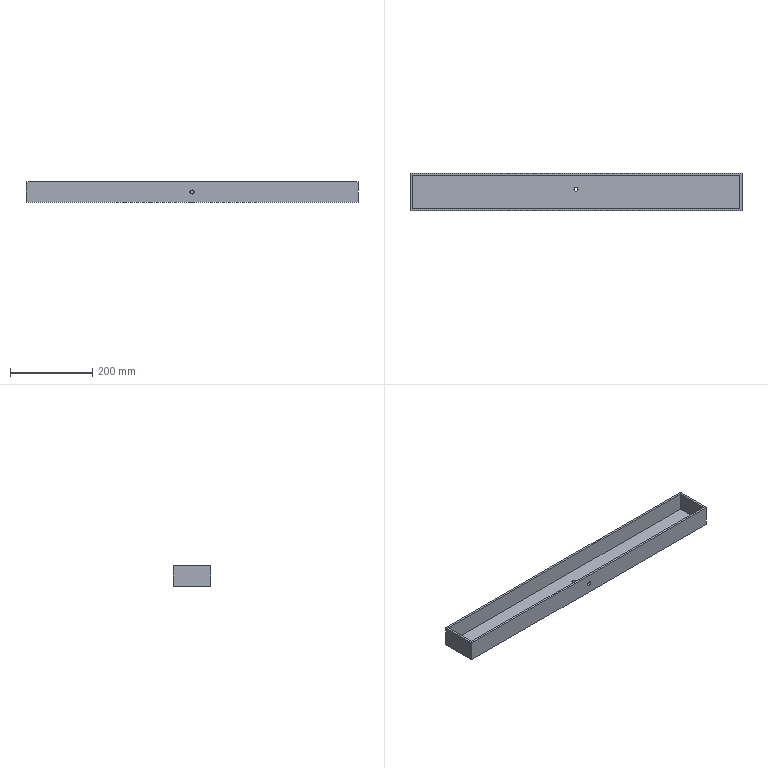Part | STEP file | 1 solid | 15 faces | box 807 x 90 x 50 mm | volume 761515 mm3 | plane 11 | cylinder 4 | commonest cylinder face diameters 10 x4
STEP:
#1=CARTESIAN_POINT('',(0.,0.,0.));
#2=DIRECTION('',(0.,0.,1.));
#3=DIRECTION('',(1.,0.,0.));
#4=AXIS2_PLACEMENT_3D('',#1,#2,#3);
#5=CARTESIAN_POINT('',(-209.535,-22.646,0.));
#6=VERTEX_POINT('',#5);
#7=CARTESIAN_POINT('',(-209.535,-22.646,5.));
#8=VERTEX_POINT('',#7);
#9=CARTESIAN_POINT('',(-209.535,-22.646,0.));
#10=DIRECTION('',(0.,0.,1.));
#11=VECTOR('',#10,1.);
#12=LINE('',#9,#11);
#13=CARTESIAN_POINT('',(-214.535,-22.646,0.));
#14=DIRECTION('',(0.,0.,1.));
#15=DIRECTION('',(1.,0.,0.));
#16=AXIS2_PLACEMENT_3D('',#13,#14,#15);
#17=CYLINDRICAL_SURFACE('',#16,5.);
#18=CARTESIAN_POINT('',(6.283,0.));
#19=DIRECTION('',(0.,1.));
#20=VECTOR('',#19,1.);
#21=LINE('',#18,#20);
#22=(GEOMETRIC_REPRESENTATION_CONTEXT(2)PARAMETRIC_REPRESENTATION_CONTEXT()REPRESENTATION_CONTEXT('',''));
#23=DEFINITIONAL_REPRESENTATION('',(#21),#22);
#24=PCURVE('',#17,#23);
#25=CARTESIAN_POINT('',(-214.535,-22.646,0.));
#26=DIRECTION('',(0.,0.,1.));
#27=DIRECTION('',(1.,0.,0.));
#28=AXIS2_PLACEMENT_3D('',#25,#26,#27);
#29=CYLINDRICAL_SURFACE('',#28,5.);
#30=CARTESIAN_POINT('',(0.,0.));
#31=DIRECTION('',(0.,1.));
#32=VECTOR('',#31,1.);
#33=LINE('',#30,#32);
#34=(GEOMETRIC_REPRESENTATION_CONTEXT(2)PARAMETRIC_REPRESENTATION_CONTEXT()REPRESENTATION_CONTEXT('',''));
#35=DEFINITIONAL_REPRESENTATION('',(#33),#34);
#36=PCURVE('',#29,#35);
#37=SURFACE_CURVE('',#12,(#24,#36),.PCURVE_S1.);
#38=EDGE_CURVE('',#6,#8,#37,.T.);
#39=ORIENTED_EDGE('',*,*,#38,.T.);
#40=CARTESIAN_POINT('',(-219.535,-22.646,5.));
#41=VERTEX_POINT('',#40);
#42=CARTESIAN_POINT('',(-214.535,-22.646,5.));
#43=DIRECTION('',(0.,0.,-1.));
#44=DIRECTION('',(1.,0.,0.));
#45=AXIS2_PLACEMENT_3D('',#42,#43,#44);
#46=CIRCLE('',#45,5.);
#47=CARTESIAN_POINT('',(6.283,5.));
#48=DIRECTION('',(-1.,0.));
#49=VECTOR('',#48,1.);
#50=LINE('',#47,#49);
#51=(GEOMETRIC_REPRESENTATION_CONTEXT(2)PARAMETRIC_REPRESENTATION_CONTEXT()REPRESENTATION_CONTEXT('',''));
#52=DEFINITIONAL_REPRESENTATION('',(#50),#51);
#53=PCURVE('',#17,#52);
#54=CARTESIAN_POINT('',(-214.535,-29.646,5.));
#55=DIRECTION('',(0.,0.,1.));
#56=DIRECTION('',(1.,0.,0.));
#57=AXIS2_PLACEMENT_3D('',#54,#55,#56);
#58=PLANE('',#57);
#59=CARTESIAN_POINT('',(5.,7.));
#60=CARTESIAN_POINT('',(5.,-1.66));
#61=CARTESIAN_POINT('',(-2.5,2.67));
#62=CARTESIAN_POINT('',(-10.,7.));
#63=CARTESIAN_POINT('',(-2.5,11.33));
#64=CARTESIAN_POINT('',(5.,15.66));
#65=CARTESIAN_POINT('',(5.,7.));
#66=(BOUNDED_CURVE()B_SPLINE_CURVE(2,(#59,#60,#61,#62,#63,#64,#65),.UNSPECIFIED.,.T.,.F.)B_SPLINE_CURVE_WITH_KNOTS((1,2,2,2,2,1),(-2.094,0.,2.094,4.189,6.283,8.378),.UNSPECIFIED.)CURVE()GEOMETRIC_REPRESENTATION_ITEM()RATIONAL_B_SPLINE_CURVE((1.,0.5,1.,0.5,1.,0.5,1.))REPRESENTATION_ITEM(''));
#67=(GEOMETRIC_REPRESENTATION_CONTEXT(2)PARAMETRIC_REPRESENTATION_CONTEXT()REPRESENTATION_CONTEXT('',''));
#68=DEFINITIONAL_REPRESENTATION('',(#66),#67);
#69=PCURVE('',#58,#68);
#70=SURFACE_CURVE('',#46,(#53,#69),.PCURVE_S1.);
#71=EDGE_CURVE('',#8,#41,#70,.T.);
#72=ORIENTED_EDGE('',*,*,#71,.T.);
#73=CARTESIAN_POINT('',(-219.535,-22.646,0.));
#74=VERTEX_POINT('',#73);
#75=CARTESIAN_POINT('',(-219.535,-22.646,0.));
#76=DIRECTION('',(0.,0.,1.));
#77=VECTOR('',#76,1.);
#78=LINE('',#75,#77);
#79=CARTESIAN_POINT('',(3.142,0.));
#80=DIRECTION('',(0.,1.));
#81=VECTOR('',#80,1.);
#82=LINE('',#79,#81);
#83=(GEOMETRIC_REPRESENTATION_CONTEXT(2)PARAMETRIC_REPRESENTATION_CONTEXT()REPRESENTATION_CONTEXT('',''));
#84=DEFINITIONAL_REPRESENTATION('',(#82),#83);
#85=PCURVE('',#17,#84);
#86=CARTESIAN_POINT('',(3.142,0.));
#87=DIRECTION('',(0.,1.));
#88=VECTOR('',#87,1.);
#89=LINE('',#86,#88);
#90=(GEOMETRIC_REPRESENTATION_CONTEXT(2)PARAMETRIC_REPRESENTATION_CONTEXT()REPRESENTATION_CONTEXT('',''));
#91=DEFINITIONAL_REPRESENTATION('',(#89),#90);
#92=PCURVE('',#29,#91);
#93=SURFACE_CURVE('',#78,(#85,#92),.PCURVE_S1.);
#94=EDGE_CURVE('',#74,#41,#93,.T.);
#95=ORIENTED_EDGE('',*,*,#94,.F.);
#96=CARTESIAN_POINT('',(-214.535,-22.646,0.));
#97=DIRECTION('',(0.,0.,-1.));
#98=DIRECTION('',(1.,0.,0.));
#99=AXIS2_PLACEMENT_3D('',#96,#97,#98);
#100=CIRCLE('',#99,5.);
#101=CARTESIAN_POINT('',(6.283,0.));
#102=DIRECTION('',(-1.,0.));
#103=VECTOR('',#102,1.);
#104=LINE('',#101,#103);
#105=(GEOMETRIC_REPRESENTATION_CONTEXT(2)PARAMETRIC_REPRESENTATION_CONTEXT()REPRESENTATION_CONTEXT('',''));
#106=DEFINITIONAL_REPRESENTATION('',(#104),#105);
#107=PCURVE('',#17,#106);
#108=CARTESIAN_POINT('',(-214.535,-29.646,0.));
#109=DIRECTION('',(0.,0.,1.));
#110=DIRECTION('',(1.,0.,0.));
#111=AXIS2_PLACEMENT_3D('',#108,#109,#110);
#112=PLANE('',#111);
#113=CARTESIAN_POINT('',(5.,7.));
#114=CARTESIAN_POINT('',(5.,-1.66));
#115=CARTESIAN_POINT('',(-2.5,2.67));
#116=CARTESIAN_POINT('',(-10.,7.));
#117=CARTESIAN_POINT('',(-2.5,11.33));
#118=CARTESIAN_POINT('',(5.,15.66));
#119=CARTESIAN_POINT('',(5.,7.));
#120=(BOUNDED_CURVE()B_SPLINE_CURVE(2,(#113,#114,#115,#116,#117,#118,#119),.UNSPECIFIED.,.T.,.F.)B_SPLINE_CURVE_WITH_KNOTS((1,2,2,2,2,1),(-2.094,0.,2.094,4.189,6.283,8.378),.UNSPECIFIED.)CURVE()GEOMETRIC_REPRESENTATION_ITEM()RATIONAL_B_SPLINE_CURVE((1.,0.5,1.,0.5,1.,0.5,1.))REPRESENTATION_ITEM(''));
#121=(GEOMETRIC_REPRESENTATION_CONTEXT(2)PARAMETRIC_REPRESENTATION_CONTEXT()REPRESENTATION_CONTEXT('',''));
#122=DEFINITIONAL_REPRESENTATION('',(#120),#121);
#123=PCURVE('',#112,#122);
#124=SURFACE_CURVE('',#100,(#107,#123),.PCURVE_S1.);
#125=EDGE_CURVE('',#6,#74,#124,.T.);
#126=ORIENTED_EDGE('',*,*,#125,.F.);
#127=EDGE_LOOP('',(#39,#72,#95,#126));
#128=FACE_BOUND('',#127,.F.);
#129=ADVANCED_FACE('',(#128),#17,.F.);
#130=CARTESIAN_POINT('',(-214.535,-74.646,30.));
#131=VERTEX_POINT('',#130);
#132=CARTESIAN_POINT('',(-214.535,-69.646,30.));
#133=VERTEX_POINT('',#132);
#134=CARTESIAN_POINT('',(-214.535,-74.646,30.));
#135=DIRECTION('',(0.,1.,0.));
#136=VECTOR('',#135,1.);
#137=LINE('',#134,#136);
#138=CARTESIAN_POINT('',(-214.535,-74.646,25.));
#139=DIRECTION('',(0.,1.,0.));
#140=DIRECTION('',(0.,0.,1.));
#141=AXIS2_PLACEMENT_3D('',#138,#139,#140);
#142=CYLINDRICAL_SURFACE('',#141,5.);
#143=CARTESIAN_POINT('',(6.283,0.));
#144=DIRECTION('',(0.,1.));
#145=VECTOR('',#144,1.);
#146=LINE('',#143,#145);
#147=(GEOMETRIC_REPRESENTATION_CONTEXT(2)PARAMETRIC_REPRESENTATION_CONTEXT()REPRESENTATION_CONTEXT('',''));
#148=DEFINITIONAL_REPRESENTATION('',(#146),#147);
#149=PCURVE('',#142,#148);
#150=CARTESIAN_POINT('',(-214.535,-74.646,25.));
#151=DIRECTION('',(0.,1.,0.));
#152=DIRECTION('',(0.,0.,1.));
#153=AXIS2_PLACEMENT_3D('',#150,#151,#152);
#154=CYLINDRICAL_SURFACE('',#153,5.);
#155=CARTESIAN_POINT('',(0.,0.));
#156=DIRECTION('',(0.,1.));
#157=VECTOR('',#156,1.);
#158=LINE('',#155,#157);
#159=(GEOMETRIC_REPRESENTATION_CONTEXT(2)PARAMETRIC_REPRESENTATION_CONTEXT()REPRESENTATION_CONTEXT('',''));
#160=DEFINITIONAL_REPRESENTATION('',(#158),#159);
#161=PCURVE('',#154,#160);
#162=SURFACE_CURVE('',#137,(#149,#161),.PCURVE_S1.);
#163=EDGE_CURVE('',#131,#133,#162,.T.);
#164=ORIENTED_EDGE('',*,*,#163,.T.);
#165=CARTESIAN_POINT('',(-214.535,-69.646,20.));
#166=VERTEX_POINT('',#165);
#167=CARTESIAN_POINT('',(-214.535,-69.646,25.));
#168=DIRECTION('',(0.,-1.,0.));
#169=DIRECTION('',(0.,0.,1.));
#170=AXIS2_PLACEMENT_3D('',#167,#168,#169);
#171=CIRCLE('',#170,5.);
#172=CARTESIAN_POINT('',(6.283,5.));
#173=DIRECTION('',(-1.,0.));
#174=VECTOR('',#173,1.);
#175=LINE('',#172,#174);
#176=(GEOMETRIC_REPRESENTATION_CONTEXT(2)PARAMETRIC_REPRESENTATION_CONTEXT()REPRESENTATION_CONTEXT('',''));
#177=DEFINITIONAL_REPRESENTATION('',(#175),#176);
#178=PCURVE('',#142,#177);
#179=CARTESIAN_POINT('',(-613.035,-69.646,0.));
#180=DIRECTION('',(0.,-1.,0.));
#181=DIRECTION('',(1.,0.,0.));
#182=AXIS2_PLACEMENT_3D('',#179,#180,#181);
#183=PLANE('',#182);
#184=CARTESIAN_POINT('',(398.5,25.));
#185=DIRECTION('',(0.,1.));
#186=AXIS2_PLACEMENT_2D('',#184,#185);
#187=CIRCLE('',#186,5.);
#188=(GEOMETRIC_REPRESENTATION_CONTEXT(2)PARAMETRIC_REPRESENTATION_CONTEXT()REPRESENTATION_CONTEXT('',''));
#189=DEFINITIONAL_REPRESENTATION('',(#187),#188);
#190=PCURVE('',#183,#189);
#191=SURFACE_CURVE('',#171,(#178,#190),.PCURVE_S1.);
#192=EDGE_CURVE('',#133,#166,#191,.T.);
#193=ORIENTED_EDGE('',*,*,#192,.T.);
#194=CARTESIAN_POINT('',(-214.535,-74.646,20.));
#195=VERTEX_POINT('',#194);
#196=CARTESIAN_POINT('',(-214.535,-74.646,20.));
#197=DIRECTION('',(0.,1.,0.));
#198=VECTOR('',#197,1.);
#199=LINE('',#196,#198);
#200=CARTESIAN_POINT('',(3.142,0.));
#201=DIRECTION('',(0.,1.));
#202=VECTOR('',#201,1.);
#203=LINE('',#200,#202);
#204=(GEOMETRIC_REPRESENTATION_CONTEXT(2)PARAMETRIC_REPRESENTATION_CONTEXT()REPRESENTATION_CONTEXT('',''));
#205=DEFINITIONAL_REPRESENTATION('',(#203),#204);
#206=PCURVE('',#142,#205);
#207=CARTESIAN_POINT('',(3.142,0.));
#208=DIRECTION('',(0.,1.));
#209=VECTOR('',#208,1.);
#210=LINE('',#207,#209);
#211=(GEOMETRIC_REPRESENTATION_CONTEXT(2)PARAMETRIC_REPRESENTATION_CONTEXT()REPRESENTATION_CONTEXT('',''));
#212=DEFINITIONAL_REPRESENTATION('',(#210),#211);
#213=PCURVE('',#154,#212);
#214=SURFACE_CURVE('',#199,(#206,#213),.PCURVE_S1.);
#215=EDGE_CURVE('',#195,#166,#214,.T.);
#216=ORIENTED_EDGE('',*,*,#215,.F.);
#217=CARTESIAN_POINT('',(-214.535,-74.646,25.));
#218=DIRECTION('',(0.,1.,0.));
#219=DIRECTION('',(0.,0.,1.));
#220=AXIS2_PLACEMENT_3D('',#217,#218,#219);
#221=CIRCLE('',#220,5.);
#222=CARTESIAN_POINT('',(0.,0.));
#223=DIRECTION('',(1.,0.));
#224=VECTOR('',#223,1.);
#225=LINE('',#222,#224);
#226=(GEOMETRIC_REPRESENTATION_CONTEXT(2)PARAMETRIC_REPRESENTATION_CONTEXT()REPRESENTATION_CONTEXT('',''));
#227=DEFINITIONAL_REPRESENTATION('',(#225),#226);
#228=PCURVE('',#142,#227);
#229=CARTESIAN_POINT('',(-618.035,-74.646,0.));
#230=DIRECTION('',(0.,-1.,0.));
#231=DIRECTION('',(1.,0.,0.));
#232=AXIS2_PLACEMENT_3D('',#229,#230,#231);
#233=PLANE('',#232);
#234=CARTESIAN_POINT('',(403.5,30.));
#235=CARTESIAN_POINT('',(412.16,30.));
#236=CARTESIAN_POINT('',(407.83,22.5));
#237=CARTESIAN_POINT('',(403.5,15.));
#238=CARTESIAN_POINT('',(399.17,22.5));
#239=CARTESIAN_POINT('',(394.84,30.));
#240=CARTESIAN_POINT('',(403.5,30.));
#241=(BOUNDED_CURVE()B_SPLINE_CURVE(2,(#234,#235,#236,#237,#238,#239,#240),.UNSPECIFIED.,.T.,.F.)B_SPLINE_CURVE_WITH_KNOTS((1,2,2,2,2,1),(-2.094,0.,2.094,4.189,6.283,8.378),.UNSPECIFIED.)CURVE()GEOMETRIC_REPRESENTATION_ITEM()RATIONAL_B_SPLINE_CURVE((1.,0.5,1.,0.5,1.,0.5,1.))REPRESENTATION_ITEM(''));
#242=(GEOMETRIC_REPRESENTATION_CONTEXT(2)PARAMETRIC_REPRESENTATION_CONTEXT()REPRESENTATION_CONTEXT('',''));
#243=DEFINITIONAL_REPRESENTATION('',(#241),#242);
#244=PCURVE('',#233,#243);
#245=SURFACE_CURVE('',#221,(#228,#244),.PCURVE_S1.);
#246=EDGE_CURVE('',#195,#131,#245,.T.);
#247=ORIENTED_EDGE('',*,*,#246,.T.);
#248=EDGE_LOOP('',(#164,#193,#216,#247));
#249=FACE_BOUND('',#248,.F.);
#250=ADVANCED_FACE('',(#249),#142,.F.);
#251=CARTESIAN_POINT('',(-618.035,15.354,0.));
#252=VERTEX_POINT('',#251);
#253=CARTESIAN_POINT('',(-618.035,-74.646,0.));
#254=VERTEX_POINT('',#253);
#255=CARTESIAN_POINT('',(-618.035,-29.646,0.));
#256=DIRECTION('',(0.,-1.,0.));
#257=VECTOR('',#256,1.);
#258=LINE('',#255,#257);
#259=CARTESIAN_POINT('',(-403.5,0.));
#260=DIRECTION('',(0.,-1.));
#261=VECTOR('',#260,1.);
#262=LINE('',#259,#261);
#263=(GEOMETRIC_REPRESENTATION_CONTEXT(2)PARAMETRIC_REPRESENTATION_CONTEXT()REPRESENTATION_CONTEXT('',''));
#264=DEFINITIONAL_REPRESENTATION('',(#262),#263);
#265=PCURVE('',#112,#264);
#266=CARTESIAN_POINT('',(-618.035,15.354,0.));
#267=DIRECTION('',(-1.,0.,0.));
#268=DIRECTION('',(0.,-1.,0.));
#269=AXIS2_PLACEMENT_3D('',#266,#267,#268);
#270=PLANE('',#269);
#271=CARTESIAN_POINT('',(45.,0.));
#272=DIRECTION('',(1.,0.));
#273=VECTOR('',#272,1.);
#274=LINE('',#271,#273);
#275=(GEOMETRIC_REPRESENTATION_CONTEXT(2)PARAMETRIC_REPRESENTATION_CONTEXT()REPRESENTATION_CONTEXT('',''));
#276=DEFINITIONAL_REPRESENTATION('',(#274),#275);
#277=PCURVE('',#270,#276);
#278=SURFACE_CURVE('',#258,(#265,#277),.PCURVE_S1.);
#279=EDGE_CURVE('',#252,#254,#278,.T.);
#280=ORIENTED_EDGE('',*,*,#279,.F.);
#281=CARTESIAN_POINT('',(188.965,15.354,0.));
#282=VERTEX_POINT('',#281);
#283=CARTESIAN_POINT('',(-214.535,15.354,0.));
#284=DIRECTION('',(-1.,0.,0.));
#285=VECTOR('',#284,1.);
#286=LINE('',#283,#285);
#287=CARTESIAN_POINT('',(0.,45.));
#288=DIRECTION('',(-1.,0.));
#289=VECTOR('',#288,1.);
#290=LINE('',#287,#289);
#291=(GEOMETRIC_REPRESENTATION_CONTEXT(2)PARAMETRIC_REPRESENTATION_CONTEXT()REPRESENTATION_CONTEXT('',''));
#292=DEFINITIONAL_REPRESENTATION('',(#290),#291);
#293=PCURVE('',#112,#292);
#294=CARTESIAN_POINT('',(188.965,15.354,0.));
#295=DIRECTION('',(0.,1.,0.));
#296=DIRECTION('',(-1.,0.,0.));
#297=AXIS2_PLACEMENT_3D('',#294,#295,#296);
#298=PLANE('',#297);
#299=CARTESIAN_POINT('',(403.5,0.));
#300=DIRECTION('',(1.,0.));
#301=VECTOR('',#300,1.);
#302=LINE('',#299,#301);
#303=(GEOMETRIC_REPRESENTATION_CONTEXT(2)PARAMETRIC_REPRESENTATION_CONTEXT()REPRESENTATION_CONTEXT('',''));
#304=DEFINITIONAL_REPRESENTATION('',(#302),#303);
#305=PCURVE('',#298,#304);
#306=SURFACE_CURVE('',#286,(#293,#305),.PCURVE_S1.);
#307=EDGE_CURVE('',#282,#252,#306,.T.);
#308=ORIENTED_EDGE('',*,*,#307,.F.);
#309=CARTESIAN_POINT('',(188.965,-74.646,0.));
#310=VERTEX_POINT('',#309);
#311=CARTESIAN_POINT('',(188.965,-29.646,0.));
#312=DIRECTION('',(0.,1.,0.));
#313=VECTOR('',#312,1.);
#314=LINE('',#311,#313);
#315=CARTESIAN_POINT('',(403.5,0.));
#316=DIRECTION('',(0.,1.));
#317=VECTOR('',#316,1.);
#318=LINE('',#315,#317);
#319=(GEOMETRIC_REPRESENTATION_CONTEXT(2)PARAMETRIC_REPRESENTATION_CONTEXT()REPRESENTATION_CONTEXT('',''));
#320=DEFINITIONAL_REPRESENTATION('',(#318),#319);
#321=PCURVE('',#112,#320);
#322=CARTESIAN_POINT('',(188.965,-74.646,0.));
#323=DIRECTION('',(1.,0.,0.));
#324=DIRECTION('',(0.,0.,-1.));
#325=AXIS2_PLACEMENT_3D('',#322,#323,#324);
#326=PLANE('',#325);
#327=CARTESIAN_POINT('',(0.,45.));
#328=DIRECTION('',(0.,1.));
#329=VECTOR('',#328,1.);
#330=LINE('',#327,#329);
#331=(GEOMETRIC_REPRESENTATION_CONTEXT(2)PARAMETRIC_REPRESENTATION_CONTEXT()REPRESENTATION_CONTEXT('',''));
#332=DEFINITIONAL_REPRESENTATION('',(#330),#331);
#333=PCURVE('',#326,#332);
#334=SURFACE_CURVE('',#314,(#321,#333),.PCURVE_S1.);
#335=EDGE_CURVE('',#310,#282,#334,.T.);
#336=ORIENTED_EDGE('',*,*,#335,.F.);
#337=CARTESIAN_POINT('',(-214.535,-74.646,0.));
#338=DIRECTION('',(1.,0.,0.));
#339=VECTOR('',#338,1.);
#340=LINE('',#337,#339);
#341=CARTESIAN_POINT('',(0.,-45.));
#342=DIRECTION('',(1.,0.));
#343=VECTOR('',#342,1.);
#344=LINE('',#341,#343);
#345=(GEOMETRIC_REPRESENTATION_CONTEXT(2)PARAMETRIC_REPRESENTATION_CONTEXT()REPRESENTATION_CONTEXT('',''));
#346=DEFINITIONAL_REPRESENTATION('',(#344),#345);
#347=PCURVE('',#112,#346);
#348=CARTESIAN_POINT('',(403.5,0.));
#349=DIRECTION('',(1.,0.));
#350=VECTOR('',#349,1.);
#351=LINE('',#348,#350);
#352=(GEOMETRIC_REPRESENTATION_CONTEXT(2)PARAMETRIC_REPRESENTATION_CONTEXT()REPRESENTATION_CONTEXT('',''));
#353=DEFINITIONAL_REPRESENTATION('',(#351),#352);
#354=PCURVE('',#233,#353);
#355=SURFACE_CURVE('',#340,(#347,#354),.PCURVE_S1.);
#356=EDGE_CURVE('',#254,#310,#355,.T.);
#357=ORIENTED_EDGE('',*,*,#356,.F.);
#358=EDGE_LOOP('',(#280,#308,#336,#357));
#359=FACE_BOUND('',#358,.T.);
#360=ORIENTED_EDGE('',*,*,#125,.F.);
#361=CARTESIAN_POINT('',(-214.535,-22.646,0.));
#362=DIRECTION('',(0.,0.,-1.));
#363=DIRECTION('',(1.,0.,0.));
#364=AXIS2_PLACEMENT_3D('',#361,#362,#363);
#365=CIRCLE('',#364,5.);
#366=CARTESIAN_POINT('',(5.,7.));
#367=CARTESIAN_POINT('',(5.,-1.66));
#368=CARTESIAN_POINT('',(-2.5,2.67));
#369=CARTESIAN_POINT('',(-10.,7.));
#370=CARTESIAN_POINT('',(-2.5,11.33));
#371=CARTESIAN_POINT('',(5.,15.66));
#372=CARTESIAN_POINT('',(5.,7.));
#373=(BOUNDED_CURVE()B_SPLINE_CURVE(2,(#366,#367,#368,#369,#370,#371,#372),.UNSPECIFIED.,.T.,.F.)B_SPLINE_CURVE_WITH_KNOTS((1,2,2,2,2,1),(-2.094,0.,2.094,4.189,6.283,8.378),.UNSPECIFIED.)CURVE()GEOMETRIC_REPRESENTATION_ITEM()RATIONAL_B_SPLINE_CURVE((1.,0.5,1.,0.5,1.,0.5,1.))REPRESENTATION_ITEM(''));
#374=(GEOMETRIC_REPRESENTATION_CONTEXT(2)PARAMETRIC_REPRESENTATION_CONTEXT()REPRESENTATION_CONTEXT('',''));
#375=DEFINITIONAL_REPRESENTATION('',(#373),#374);
#376=PCURVE('',#112,#375);
#377=CARTESIAN_POINT('',(6.283,0.));
#378=DIRECTION('',(-1.,0.));
#379=VECTOR('',#378,1.);
#380=LINE('',#377,#379);
#381=(GEOMETRIC_REPRESENTATION_CONTEXT(2)PARAMETRIC_REPRESENTATION_CONTEXT()REPRESENTATION_CONTEXT('',''));
#382=DEFINITIONAL_REPRESENTATION('',(#380),#381);
#383=PCURVE('',#29,#382);
#384=SURFACE_CURVE('',#365,(#376,#383),.PCURVE_S1.);
#385=EDGE_CURVE('',#74,#6,#384,.T.);
#386=ORIENTED_EDGE('',*,*,#385,.F.);
#387=EDGE_LOOP('',(#360,#386));
#388=FACE_BOUND('',#387,.T.);
#389=ADVANCED_FACE('',(#359,#388),#112,.F.);
#390=CARTESIAN_POINT('',(188.965,-74.646,50.));
#391=VERTEX_POINT('',#390);
#392=CARTESIAN_POINT('',(-618.035,-74.646,50.));
#393=VERTEX_POINT('',#392);
#394=CARTESIAN_POINT('',(-618.035,-74.646,50.));
#395=DIRECTION('',(-1.,0.,0.));
#396=VECTOR('',#395,1.);
#397=LINE('',#394,#396);
#398=CARTESIAN_POINT('',(0.,50.));
#399=DIRECTION('',(-1.,0.));
#400=VECTOR('',#399,1.);
#401=LINE('',#398,#400);
#402=(GEOMETRIC_REPRESENTATION_CONTEXT(2)PARAMETRIC_REPRESENTATION_CONTEXT()REPRESENTATION_CONTEXT('',''));
#403=DEFINITIONAL_REPRESENTATION('',(#401),#402);
#404=PCURVE('',#233,#403);
#405=CARTESIAN_POINT('',(-214.535,-29.646,50.));
#406=DIRECTION('',(0.,0.,1.));
#407=DIRECTION('',(1.,0.,0.));
#408=AXIS2_PLACEMENT_3D('',#405,#406,#407);
#409=PLANE('',#408);
#410=CARTESIAN_POINT('',(-403.5,-45.));
#411=DIRECTION('',(-1.,0.));
#412=VECTOR('',#411,1.);
#413=LINE('',#410,#412);
#414=(GEOMETRIC_REPRESENTATION_CONTEXT(2)PARAMETRIC_REPRESENTATION_CONTEXT()REPRESENTATION_CONTEXT('',''));
#415=DEFINITIONAL_REPRESENTATION('',(#413),#414);
#416=PCURVE('',#409,#415);
#417=SURFACE_CURVE('',#397,(#404,#416),.PCURVE_S1.);
#418=EDGE_CURVE('',#391,#393,#417,.T.);
#419=ORIENTED_EDGE('',*,*,#418,.T.);
#420=CARTESIAN_POINT('',(-618.035,-74.646,0.));
#421=DIRECTION('',(0.,0.,-1.));
#422=VECTOR('',#421,1.);
#423=LINE('',#420,#422);
#424=CARTESIAN_POINT('',(0.,0.));
#425=DIRECTION('',(0.,-1.));
#426=VECTOR('',#425,1.);
#427=LINE('',#424,#426);
#428=(GEOMETRIC_REPRESENTATION_CONTEXT(2)PARAMETRIC_REPRESENTATION_CONTEXT()REPRESENTATION_CONTEXT('',''));
#429=DEFINITIONAL_REPRESENTATION('',(#427),#428);
#430=PCURVE('',#233,#429);
#431=CARTESIAN_POINT('',(90.,0.));
#432=DIRECTION('',(0.,-1.));
#433=VECTOR('',#432,1.);
#434=LINE('',#431,#433);
#435=(GEOMETRIC_REPRESENTATION_CONTEXT(2)PARAMETRIC_REPRESENTATION_CONTEXT()REPRESENTATION_CONTEXT('',''));
#436=DEFINITIONAL_REPRESENTATION('',(#434),#435);
#437=PCURVE('',#270,#436);
#438=SURFACE_CURVE('',#423,(#430,#437),.PCURVE_S1.);
#439=EDGE_CURVE('',#393,#254,#438,.T.);
#440=ORIENTED_EDGE('',*,*,#439,.T.);
#441=ORIENTED_EDGE('',*,*,#356,.T.);
#442=CARTESIAN_POINT('',(188.965,-74.646,0.));
#443=DIRECTION('',(0.,0.,1.));
#444=VECTOR('',#443,1.);
#445=LINE('',#442,#444);
#446=CARTESIAN_POINT('',(807.,0.));
#447=DIRECTION('',(0.,1.));
#448=VECTOR('',#447,1.);
#449=LINE('',#446,#448);
#450=(GEOMETRIC_REPRESENTATION_CONTEXT(2)PARAMETRIC_REPRESENTATION_CONTEXT()REPRESENTATION_CONTEXT('',''));
#451=DEFINITIONAL_REPRESENTATION('',(#449),#450);
#452=PCURVE('',#233,#451);
#453=CARTESIAN_POINT('',(0.,0.));
#454=DIRECTION('',(-1.,0.));
#455=VECTOR('',#454,1.);
#456=LINE('',#453,#455);
#457=(GEOMETRIC_REPRESENTATION_CONTEXT(2)PARAMETRIC_REPRESENTATION_CONTEXT()REPRESENTATION_CONTEXT('',''));
#458=DEFINITIONAL_REPRESENTATION('',(#456),#457);
#459=PCURVE('',#326,#458);
#460=SURFACE_CURVE('',#445,(#452,#459),.PCURVE_S1.);
#461=EDGE_CURVE('',#310,#391,#460,.T.);
#462=ORIENTED_EDGE('',*,*,#461,.T.);
#463=EDGE_LOOP('',(#419,#440,#441,#462));
#464=FACE_BOUND('',#463,.T.);
#465=CARTESIAN_POINT('',(-214.535,-74.646,25.));
#466=DIRECTION('',(0.,1.,0.));
#467=DIRECTION('',(0.,0.,1.));
#468=AXIS2_PLACEMENT_3D('',#465,#466,#467);
#469=CIRCLE('',#468,5.);
#470=CARTESIAN_POINT('',(403.5,30.));
#471=CARTESIAN_POINT('',(412.16,30.));
#472=CARTESIAN_POINT('',(407.83,22.5));
#473=CARTESIAN_POINT('',(403.5,15.));
#474=CARTESIAN_POINT('',(399.17,22.5));
#475=CARTESIAN_POINT('',(394.84,30.));
#476=CARTESIAN_POINT('',(403.5,30.));
#477=(BOUNDED_CURVE()B_SPLINE_CURVE(2,(#470,#471,#472,#473,#474,#475,#476),.UNSPECIFIED.,.T.,.F.)B_SPLINE_CURVE_WITH_KNOTS((1,2,2,2,2,1),(-2.094,0.,2.094,4.189,6.283,8.378),.UNSPECIFIED.)CURVE()GEOMETRIC_REPRESENTATION_ITEM()RATIONAL_B_SPLINE_CURVE((1.,0.5,1.,0.5,1.,0.5,1.))REPRESENTATION_ITEM(''));
#478=(GEOMETRIC_REPRESENTATION_CONTEXT(2)PARAMETRIC_REPRESENTATION_CONTEXT()REPRESENTATION_CONTEXT('',''));
#479=DEFINITIONAL_REPRESENTATION('',(#477),#478);
#480=PCURVE('',#233,#479);
#481=CARTESIAN_POINT('',(0.,0.));
#482=DIRECTION('',(1.,0.));
#483=VECTOR('',#482,1.);
#484=LINE('',#481,#483);
#485=(GEOMETRIC_REPRESENTATION_CONTEXT(2)PARAMETRIC_REPRESENTATION_CONTEXT()REPRESENTATION_CONTEXT('',''));
#486=DEFINITIONAL_REPRESENTATION('',(#484),#485);
#487=PCURVE('',#154,#486);
#488=SURFACE_CURVE('',#469,(#480,#487),.PCURVE_S1.);
#489=EDGE_CURVE('',#131,#195,#488,.T.);
#490=ORIENTED_EDGE('',*,*,#489,.T.);
#491=ORIENTED_EDGE('',*,*,#246,.T.);
#492=EDGE_LOOP('',(#490,#491));
#493=FACE_BOUND('',#492,.T.);
#494=ADVANCED_FACE('',(#464,#493),#233,.T.);
#495=CARTESIAN_POINT('',(-618.035,15.354,50.));
#496=VERTEX_POINT('',#495);
#497=CARTESIAN_POINT('',(-618.035,15.354,50.));
#498=DIRECTION('',(0.,1.,0.));
#499=VECTOR('',#498,1.);
#500=LINE('',#497,#499);
#501=CARTESIAN_POINT('',(0.,50.));
#502=DIRECTION('',(-1.,0.));
#503=VECTOR('',#502,1.);
#504=LINE('',#501,#503);
#505=(GEOMETRIC_REPRESENTATION_CONTEXT(2)PARAMETRIC_REPRESENTATION_CONTEXT()REPRESENTATION_CONTEXT('',''));
#506=DEFINITIONAL_REPRESENTATION('',(#504),#505);
#507=PCURVE('',#270,#506);
#508=CARTESIAN_POINT('',(-403.5,45.));
#509=DIRECTION('',(0.,1.));
#510=VECTOR('',#509,1.);
#511=LINE('',#508,#510);
#512=(GEOMETRIC_REPRESENTATION_CONTEXT(2)PARAMETRIC_REPRESENTATION_CONTEXT()REPRESENTATION_CONTEXT('',''));
#513=DEFINITIONAL_REPRESENTATION('',(#511),#512);
#514=PCURVE('',#409,#513);
#515=SURFACE_CURVE('',#500,(#507,#514),.PCURVE_S1.);
#516=EDGE_CURVE('',#393,#496,#515,.T.);
#517=ORIENTED_EDGE('',*,*,#516,.T.);
#518=CARTESIAN_POINT('',(-618.035,15.354,0.));
#519=DIRECTION('',(0.,0.,-1.));
#520=VECTOR('',#519,1.);
#521=LINE('',#518,#520);
#522=CARTESIAN_POINT('',(0.,0.));
#523=DIRECTION('',(0.,-1.));
#524=VECTOR('',#523,1.);
#525=LINE('',#522,#524);
#526=(GEOMETRIC_REPRESENTATION_CONTEXT(2)PARAMETRIC_REPRESENTATION_CONTEXT()REPRESENTATION_CONTEXT('',''));
#527=DEFINITIONAL_REPRESENTATION('',(#525),#526);
#528=PCURVE('',#270,#527);
#529=CARTESIAN_POINT('',(807.,0.));
#530=DIRECTION('',(0.,-1.));
#531=VECTOR('',#530,1.);
#532=LINE('',#529,#531);
#533=(GEOMETRIC_REPRESENTATION_CONTEXT(2)PARAMETRIC_REPRESENTATION_CONTEXT()REPRESENTATION_CONTEXT('',''));
#534=DEFINITIONAL_REPRESENTATION('',(#532),#533);
#535=PCURVE('',#298,#534);
#536=SURFACE_CURVE('',#521,(#528,#535),.PCURVE_S1.);
#537=EDGE_CURVE('',#496,#252,#536,.T.);
#538=ORIENTED_EDGE('',*,*,#537,.T.);
#539=ORIENTED_EDGE('',*,*,#279,.T.);
#540=ORIENTED_EDGE('',*,*,#439,.F.);
#541=EDGE_LOOP('',(#517,#538,#539,#540));
#542=FACE_BOUND('',#541,.T.);
#543=ADVANCED_FACE('',(#542),#270,.T.);
#544=CARTESIAN_POINT('',(188.965,15.354,50.));
#545=VERTEX_POINT('',#544);
#546=CARTESIAN_POINT('',(188.965,15.354,50.));
#547=DIRECTION('',(1.,0.,0.));
#548=VECTOR('',#547,1.);
#549=LINE('',#546,#548);
#550=CARTESIAN_POINT('',(0.,50.));
#551=DIRECTION('',(-1.,0.));
#552=VECTOR('',#551,1.);
#553=LINE('',#550,#552);
#554=(GEOMETRIC_REPRESENTATION_CONTEXT(2)PARAMETRIC_REPRESENTATION_CONTEXT()REPRESENTATION_CONTEXT('',''));
#555=DEFINITIONAL_REPRESENTATION('',(#553),#554);
#556=PCURVE('',#298,#555);
#557=CARTESIAN_POINT('',(403.5,45.));
#558=DIRECTION('',(1.,0.));
#559=VECTOR('',#558,1.);
#560=LINE('',#557,#559);
#561=(GEOMETRIC_REPRESENTATION_CONTEXT(2)PARAMETRIC_REPRESENTATION_CONTEXT()REPRESENTATION_CONTEXT('',''));
#562=DEFINITIONAL_REPRESENTATION('',(#560),#561);
#563=PCURVE('',#409,#562);
#564=SURFACE_CURVE('',#549,(#556,#563),.PCURVE_S1.);
#565=EDGE_CURVE('',#496,#545,#564,.T.);
#566=ORIENTED_EDGE('',*,*,#565,.T.);
#567=CARTESIAN_POINT('',(188.965,15.354,0.));
#568=DIRECTION('',(0.,0.,-1.));
#569=VECTOR('',#568,1.);
#570=LINE('',#567,#569);
#571=CARTESIAN_POINT('',(0.,0.));
#572=DIRECTION('',(0.,-1.));
#573=VECTOR('',#572,1.);
#574=LINE('',#571,#573);
#575=(GEOMETRIC_REPRESENTATION_CONTEXT(2)PARAMETRIC_REPRESENTATION_CONTEXT()REPRESENTATION_CONTEXT('',''));
#576=DEFINITIONAL_REPRESENTATION('',(#574),#575);
#577=PCURVE('',#298,#576);
#578=CARTESIAN_POINT('',(0.,90.));
#579=DIRECTION('',(1.,0.));
#580=VECTOR('',#579,1.);
#581=LINE('',#578,#580);
#582=(GEOMETRIC_REPRESENTATION_CONTEXT(2)PARAMETRIC_REPRESENTATION_CONTEXT()REPRESENTATION_CONTEXT('',''));
#583=DEFINITIONAL_REPRESENTATION('',(#581),#582);
#584=PCURVE('',#326,#583);
#585=SURFACE_CURVE('',#570,(#577,#584),.PCURVE_S1.);
#586=EDGE_CURVE('',#545,#282,#585,.T.);
#587=ORIENTED_EDGE('',*,*,#586,.T.);
#588=ORIENTED_EDGE('',*,*,#307,.T.);
#589=ORIENTED_EDGE('',*,*,#537,.F.);
#590=EDGE_LOOP('',(#566,#587,#588,#589));
#591=FACE_BOUND('',#590,.T.);
#592=ADVANCED_FACE('',(#591),#298,.T.);
#593=CARTESIAN_POINT('',(188.965,-74.646,50.));
#594=DIRECTION('',(0.,-1.,0.));
#595=VECTOR('',#594,1.);
#596=LINE('',#593,#595);
#597=CARTESIAN_POINT('',(-50.,0.));
#598=DIRECTION('',(0.,-1.));
#599=VECTOR('',#598,1.);
#600=LINE('',#597,#599);
#601=(GEOMETRIC_REPRESENTATION_CONTEXT(2)PARAMETRIC_REPRESENTATION_CONTEXT()REPRESENTATION_CONTEXT('',''));
#602=DEFINITIONAL_REPRESENTATION('',(#600),#601);
#603=PCURVE('',#326,#602);
#604=CARTESIAN_POINT('',(403.5,-45.));
#605=DIRECTION('',(0.,-1.));
#606=VECTOR('',#605,1.);
#607=LINE('',#604,#606);
#608=(GEOMETRIC_REPRESENTATION_CONTEXT(2)PARAMETRIC_REPRESENTATION_CONTEXT()REPRESENTATION_CONTEXT('',''));
#609=DEFINITIONAL_REPRESENTATION('',(#607),#608);
#610=PCURVE('',#409,#609);
#611=SURFACE_CURVE('',#596,(#603,#610),.PCURVE_S1.);
#612=EDGE_CURVE('',#545,#391,#611,.T.);
#613=ORIENTED_EDGE('',*,*,#612,.T.);
#614=ORIENTED_EDGE('',*,*,#461,.F.);
#615=ORIENTED_EDGE('',*,*,#335,.T.);
#616=ORIENTED_EDGE('',*,*,#586,.F.);
#617=EDGE_LOOP('',(#613,#614,#615,#616));
#618=FACE_BOUND('',#617,.T.);
#619=ADVANCED_FACE('',(#618),#326,.T.);
#620=CARTESIAN_POINT('',(-214.535,-22.646,5.));
#621=DIRECTION('',(0.,0.,-1.));
#622=DIRECTION('',(1.,0.,0.));
#623=AXIS2_PLACEMENT_3D('',#620,#621,#622);
#624=CIRCLE('',#623,5.);
#625=CARTESIAN_POINT('',(6.283,5.));
#626=DIRECTION('',(-1.,0.));
#627=VECTOR('',#626,1.);
#628=LINE('',#625,#627);
#629=(GEOMETRIC_REPRESENTATION_CONTEXT(2)PARAMETRIC_REPRESENTATION_CONTEXT()REPRESENTATION_CONTEXT('',''));
#630=DEFINITIONAL_REPRESENTATION('',(#628),#629);
#631=PCURVE('',#29,#630);
#632=CARTESIAN_POINT('',(5.,7.));
#633=CARTESIAN_POINT('',(5.,-1.66));
#634=CARTESIAN_POINT('',(-2.5,2.67));
#635=CARTESIAN_POINT('',(-10.,7.));
#636=CARTESIAN_POINT('',(-2.5,11.33));
#637=CARTESIAN_POINT('',(5.,15.66));
#638=CARTESIAN_POINT('',(5.,7.));
#639=(BOUNDED_CURVE()B_SPLINE_CURVE(2,(#632,#633,#634,#635,#636,#637,#638),.UNSPECIFIED.,.T.,.F.)B_SPLINE_CURVE_WITH_KNOTS((1,2,2,2,2,1),(-2.094,0.,2.094,4.189,6.283,8.378),.UNSPECIFIED.)CURVE()GEOMETRIC_REPRESENTATION_ITEM()RATIONAL_B_SPLINE_CURVE((1.,0.5,1.,0.5,1.,0.5,1.))REPRESENTATION_ITEM(''));
#640=(GEOMETRIC_REPRESENTATION_CONTEXT(2)PARAMETRIC_REPRESENTATION_CONTEXT()REPRESENTATION_CONTEXT('',''));
#641=DEFINITIONAL_REPRESENTATION('',(#639),#640);
#642=PCURVE('',#58,#641);
#643=SURFACE_CURVE('',#624,(#631,#642),.PCURVE_S1.);
#644=EDGE_CURVE('',#41,#8,#643,.T.);
#645=ORIENTED_EDGE('',*,*,#644,.T.);
#646=ORIENTED_EDGE('',*,*,#38,.F.);
#647=ORIENTED_EDGE('',*,*,#385,.F.);
#648=ORIENTED_EDGE('',*,*,#94,.T.);
#649=EDGE_LOOP('',(#645,#646,#647,#648));
#650=FACE_BOUND('',#649,.F.);
#651=ADVANCED_FACE('',(#650),#29,.F.);
#652=ORIENTED_EDGE('',*,*,#565,.F.);
#653=ORIENTED_EDGE('',*,*,#516,.F.);
#654=ORIENTED_EDGE('',*,*,#418,.F.);
#655=ORIENTED_EDGE('',*,*,#612,.F.);
#656=EDGE_LOOP('',(#652,#653,#654,#655));
#657=FACE_BOUND('',#656,.T.);
#658=CARTESIAN_POINT('',(-613.035,-69.646,50.));
#659=VERTEX_POINT('',#658);
#660=CARTESIAN_POINT('',(-613.035,10.354,50.));
#661=VERTEX_POINT('',#660);
#662=CARTESIAN_POINT('',(-613.035,-29.646,50.));
#663=DIRECTION('',(0.,1.,0.));
#664=VECTOR('',#663,1.);
#665=LINE('',#662,#664);
#666=CARTESIAN_POINT('',(-398.5,0.));
#667=DIRECTION('',(0.,1.));
#668=VECTOR('',#667,1.);
#669=LINE('',#666,#668);
#670=(GEOMETRIC_REPRESENTATION_CONTEXT(2)PARAMETRIC_REPRESENTATION_CONTEXT()REPRESENTATION_CONTEXT('',''));
#671=DEFINITIONAL_REPRESENTATION('',(#669),#670);
#672=PCURVE('',#409,#671);
#673=CARTESIAN_POINT('',(-613.035,10.354,0.));
#674=DIRECTION('',(-1.,0.,0.));
#675=DIRECTION('',(0.,0.,1.));
#676=AXIS2_PLACEMENT_3D('',#673,#674,#675);
#677=PLANE('',#676);
#678=CARTESIAN_POINT('',(50.,-40.));
#679=DIRECTION('',(0.,1.));
#680=VECTOR('',#679,1.);
#681=LINE('',#678,#680);
#682=(GEOMETRIC_REPRESENTATION_CONTEXT(2)PARAMETRIC_REPRESENTATION_CONTEXT()REPRESENTATION_CONTEXT('',''));
#683=DEFINITIONAL_REPRESENTATION('',(#681),#682);
#684=PCURVE('',#677,#683);
#685=SURFACE_CURVE('',#665,(#672,#684),.PCURVE_S1.);
#686=EDGE_CURVE('',#659,#661,#685,.T.);
#687=ORIENTED_EDGE('',*,*,#686,.T.);
#688=CARTESIAN_POINT('',(183.965,10.354,50.));
#689=VERTEX_POINT('',#688);
#690=CARTESIAN_POINT('',(-214.535,10.354,50.));
#691=DIRECTION('',(1.,0.,0.));
#692=VECTOR('',#691,1.);
#693=LINE('',#690,#692);
#694=CARTESIAN_POINT('',(0.,40.));
#695=DIRECTION('',(1.,0.));
#696=VECTOR('',#695,1.);
#697=LINE('',#694,#696);
#698=(GEOMETRIC_REPRESENTATION_CONTEXT(2)PARAMETRIC_REPRESENTATION_CONTEXT()REPRESENTATION_CONTEXT('',''));
#699=DEFINITIONAL_REPRESENTATION('',(#697),#698);
#700=PCURVE('',#409,#699);
#701=CARTESIAN_POINT('',(183.965,10.354,0.));
#702=DIRECTION('',(0.,1.,0.));
#703=DIRECTION('',(-1.,0.,0.));
#704=AXIS2_PLACEMENT_3D('',#701,#702,#703);
#705=PLANE('',#704);
#706=CARTESIAN_POINT('',(398.5,50.));
#707=DIRECTION('',(-1.,0.));
#708=VECTOR('',#707,1.);
#709=LINE('',#706,#708);
#710=(GEOMETRIC_REPRESENTATION_CONTEXT(2)PARAMETRIC_REPRESENTATION_CONTEXT()REPRESENTATION_CONTEXT('',''));
#711=DEFINITIONAL_REPRESENTATION('',(#709),#710);
#712=PCURVE('',#705,#711);
#713=SURFACE_CURVE('',#693,(#700,#712),.PCURVE_S1.);
#714=EDGE_CURVE('',#661,#689,#713,.T.);
#715=ORIENTED_EDGE('',*,*,#714,.T.);
#716=CARTESIAN_POINT('',(183.965,-69.646,50.));
#717=VERTEX_POINT('',#716);
#718=CARTESIAN_POINT('',(183.965,-29.646,50.));
#719=DIRECTION('',(0.,-1.,0.));
#720=VECTOR('',#719,1.);
#721=LINE('',#718,#720);
#722=CARTESIAN_POINT('',(398.5,0.));
#723=DIRECTION('',(0.,-1.));
#724=VECTOR('',#723,1.);
#725=LINE('',#722,#724);
#726=(GEOMETRIC_REPRESENTATION_CONTEXT(2)PARAMETRIC_REPRESENTATION_CONTEXT()REPRESENTATION_CONTEXT('',''));
#727=DEFINITIONAL_REPRESENTATION('',(#725),#726);
#728=PCURVE('',#409,#727);
#729=CARTESIAN_POINT('',(183.965,-69.646,0.));
#730=DIRECTION('',(1.,0.,0.));
#731=DIRECTION('',(0.,0.,-1.));
#732=AXIS2_PLACEMENT_3D('',#729,#730,#731);
#733=PLANE('',#732);
#734=CARTESIAN_POINT('',(-50.,40.));
#735=DIRECTION('',(0.,-1.));
#736=VECTOR('',#735,1.);
#737=LINE('',#734,#736);
#738=(GEOMETRIC_REPRESENTATION_CONTEXT(2)PARAMETRIC_REPRESENTATION_CONTEXT()REPRESENTATION_CONTEXT('',''));
#739=DEFINITIONAL_REPRESENTATION('',(#737),#738);
#740=PCURVE('',#733,#739);
#741=SURFACE_CURVE('',#721,(#728,#740),.PCURVE_S1.);
#742=EDGE_CURVE('',#689,#717,#741,.T.);
#743=ORIENTED_EDGE('',*,*,#742,.T.);
#744=CARTESIAN_POINT('',(-214.535,-69.646,50.));
#745=DIRECTION('',(-1.,0.,0.));
#746=VECTOR('',#745,1.);
#747=LINE('',#744,#746);
#748=CARTESIAN_POINT('',(0.,-40.));
#749=DIRECTION('',(-1.,0.));
#750=VECTOR('',#749,1.);
#751=LINE('',#748,#750);
#752=(GEOMETRIC_REPRESENTATION_CONTEXT(2)PARAMETRIC_REPRESENTATION_CONTEXT()REPRESENTATION_CONTEXT('',''));
#753=DEFINITIONAL_REPRESENTATION('',(#751),#752);
#754=PCURVE('',#409,#753);
#755=CARTESIAN_POINT('',(398.5,50.));
#756=DIRECTION('',(-1.,0.));
#757=VECTOR('',#756,1.);
#758=LINE('',#755,#757);
#759=(GEOMETRIC_REPRESENTATION_CONTEXT(2)PARAMETRIC_REPRESENTATION_CONTEXT()REPRESENTATION_CONTEXT('',''));
#760=DEFINITIONAL_REPRESENTATION('',(#758),#759);
#761=PCURVE('',#183,#760);
#762=SURFACE_CURVE('',#747,(#754,#761),.PCURVE_S1.);
#763=EDGE_CURVE('',#717,#659,#762,.T.);
#764=ORIENTED_EDGE('',*,*,#763,.T.);
#765=EDGE_LOOP('',(#687,#715,#743,#764));
#766=FACE_BOUND('',#765,.T.);
#767=ADVANCED_FACE('',(#657,#766),#409,.T.);
#768=CARTESIAN_POINT('',(-214.535,-69.646,25.));
#769=DIRECTION('',(0.,-1.,0.));
#770=DIRECTION('',(0.,0.,1.));
#771=AXIS2_PLACEMENT_3D('',#768,#769,#770);
#772=CIRCLE('',#771,5.);
#773=CARTESIAN_POINT('',(6.283,5.));
#774=DIRECTION('',(-1.,0.));
#775=VECTOR('',#774,1.);
#776=LINE('',#773,#775);
#777=(GEOMETRIC_REPRESENTATION_CONTEXT(2)PARAMETRIC_REPRESENTATION_CONTEXT()REPRESENTATION_CONTEXT('',''));
#778=DEFINITIONAL_REPRESENTATION('',(#776),#777);
#779=PCURVE('',#154,#778);
#780=CARTESIAN_POINT('',(398.5,25.));
#781=DIRECTION('',(0.,1.));
#782=AXIS2_PLACEMENT_2D('',#780,#781);
#783=CIRCLE('',#782,5.);
#784=(GEOMETRIC_REPRESENTATION_CONTEXT(2)PARAMETRIC_REPRESENTATION_CONTEXT()REPRESENTATION_CONTEXT('',''));
#785=DEFINITIONAL_REPRESENTATION('',(#783),#784);
#786=PCURVE('',#183,#785);
#787=SURFACE_CURVE('',#772,(#779,#786),.PCURVE_S1.);
#788=EDGE_CURVE('',#166,#133,#787,.T.);
#789=ORIENTED_EDGE('',*,*,#788,.T.);
#790=ORIENTED_EDGE('',*,*,#163,.F.);
#791=ORIENTED_EDGE('',*,*,#489,.T.);
#792=ORIENTED_EDGE('',*,*,#215,.T.);
#793=EDGE_LOOP('',(#789,#790,#791,#792));
#794=FACE_BOUND('',#793,.F.);
#795=ADVANCED_FACE('',(#794),#154,.F.);
#796=CARTESIAN_POINT('',(-613.035,-69.646,5.));
#797=VERTEX_POINT('',#796);
#798=CARTESIAN_POINT('',(183.965,-69.646,5.));
#799=VERTEX_POINT('',#798);
#800=CARTESIAN_POINT('',(-214.535,-69.646,5.));
#801=DIRECTION('',(1.,0.,0.));
#802=VECTOR('',#801,1.);
#803=LINE('',#800,#802);
#804=CARTESIAN_POINT('',(0.,-40.));
#805=DIRECTION('',(1.,0.));
#806=VECTOR('',#805,1.);
#807=LINE('',#804,#806);
#808=(GEOMETRIC_REPRESENTATION_CONTEXT(2)PARAMETRIC_REPRESENTATION_CONTEXT()REPRESENTATION_CONTEXT('',''));
#809=DEFINITIONAL_REPRESENTATION('',(#807),#808);
#810=PCURVE('',#58,#809);
#811=CARTESIAN_POINT('',(398.5,5.));
#812=DIRECTION('',(1.,0.));
#813=VECTOR('',#812,1.);
#814=LINE('',#811,#813);
#815=(GEOMETRIC_REPRESENTATION_CONTEXT(2)PARAMETRIC_REPRESENTATION_CONTEXT()REPRESENTATION_CONTEXT('',''));
#816=DEFINITIONAL_REPRESENTATION('',(#814),#815);
#817=PCURVE('',#183,#816);
#818=SURFACE_CURVE('',#803,(#810,#817),.PCURVE_S1.);
#819=EDGE_CURVE('',#797,#799,#818,.T.);
#820=ORIENTED_EDGE('',*,*,#819,.T.);
#821=CARTESIAN_POINT('',(183.965,10.354,5.));
#822=VERTEX_POINT('',#821);
#823=CARTESIAN_POINT('',(183.965,-29.646,5.));
#824=DIRECTION('',(0.,1.,0.));
#825=VECTOR('',#824,1.);
#826=LINE('',#823,#825);
#827=CARTESIAN_POINT('',(398.5,0.));
#828=DIRECTION('',(0.,1.));
#829=VECTOR('',#828,1.);
#830=LINE('',#827,#829);
#831=(GEOMETRIC_REPRESENTATION_CONTEXT(2)PARAMETRIC_REPRESENTATION_CONTEXT()REPRESENTATION_CONTEXT('',''));
#832=DEFINITIONAL_REPRESENTATION('',(#830),#831);
#833=PCURVE('',#58,#832);
#834=CARTESIAN_POINT('',(-5.,40.));
#835=DIRECTION('',(0.,1.));
#836=VECTOR('',#835,1.);
#837=LINE('',#834,#836);
#838=(GEOMETRIC_REPRESENTATION_CONTEXT(2)PARAMETRIC_REPRESENTATION_CONTEXT()REPRESENTATION_CONTEXT('',''));
#839=DEFINITIONAL_REPRESENTATION('',(#837),#838);
#840=PCURVE('',#733,#839);
#841=SURFACE_CURVE('',#826,(#833,#840),.PCURVE_S1.);
#842=EDGE_CURVE('',#799,#822,#841,.T.);
#843=ORIENTED_EDGE('',*,*,#842,.T.);
#844=CARTESIAN_POINT('',(-613.035,10.354,5.));
#845=VERTEX_POINT('',#844);
#846=CARTESIAN_POINT('',(-214.535,10.354,5.));
#847=DIRECTION('',(-1.,0.,0.));
#848=VECTOR('',#847,1.);
#849=LINE('',#846,#848);
#850=CARTESIAN_POINT('',(0.,40.));
#851=DIRECTION('',(-1.,0.));
#852=VECTOR('',#851,1.);
#853=LINE('',#850,#852);
#854=(GEOMETRIC_REPRESENTATION_CONTEXT(2)PARAMETRIC_REPRESENTATION_CONTEXT()REPRESENTATION_CONTEXT('',''));
#855=DEFINITIONAL_REPRESENTATION('',(#853),#854);
#856=PCURVE('',#58,#855);
#857=CARTESIAN_POINT('',(398.5,5.));
#858=DIRECTION('',(1.,0.));
#859=VECTOR('',#858,1.);
#860=LINE('',#857,#859);
#861=(GEOMETRIC_REPRESENTATION_CONTEXT(2)PARAMETRIC_REPRESENTATION_CONTEXT()REPRESENTATION_CONTEXT('',''));
#862=DEFINITIONAL_REPRESENTATION('',(#860),#861);
#863=PCURVE('',#705,#862);
#864=SURFACE_CURVE('',#849,(#856,#863),.PCURVE_S1.);
#865=EDGE_CURVE('',#822,#845,#864,.T.);
#866=ORIENTED_EDGE('',*,*,#865,.T.);
#867=CARTESIAN_POINT('',(-613.035,-29.646,5.));
#868=DIRECTION('',(0.,-1.,0.));
#869=VECTOR('',#868,1.);
#870=LINE('',#867,#869);
#871=CARTESIAN_POINT('',(-398.5,0.));
#872=DIRECTION('',(0.,-1.));
#873=VECTOR('',#872,1.);
#874=LINE('',#871,#873);
#875=(GEOMETRIC_REPRESENTATION_CONTEXT(2)PARAMETRIC_REPRESENTATION_CONTEXT()REPRESENTATION_CONTEXT('',''));
#876=DEFINITIONAL_REPRESENTATION('',(#874),#875);
#877=PCURVE('',#58,#876);
#878=CARTESIAN_POINT('',(5.,-40.));
#879=DIRECTION('',(0.,-1.));
#880=VECTOR('',#879,1.);
#881=LINE('',#878,#880);
#882=(GEOMETRIC_REPRESENTATION_CONTEXT(2)PARAMETRIC_REPRESENTATION_CONTEXT()REPRESENTATION_CONTEXT('',''));
#883=DEFINITIONAL_REPRESENTATION('',(#881),#882);
#884=PCURVE('',#677,#883);
#885=SURFACE_CURVE('',#870,(#877,#884),.PCURVE_S1.);
#886=EDGE_CURVE('',#845,#797,#885,.T.);
#887=ORIENTED_EDGE('',*,*,#886,.T.);
#888=EDGE_LOOP('',(#820,#843,#866,#887));
#889=FACE_BOUND('',#888,.T.);
#890=ORIENTED_EDGE('',*,*,#71,.T.);
#891=ORIENTED_EDGE('',*,*,#644,.T.);
#892=EDGE_LOOP('',(#890,#891));
#893=FACE_BOUND('',#892,.T.);
#894=ADVANCED_FACE('',(#889,#893),#58,.T.);
#895=CARTESIAN_POINT('',(183.965,10.354,0.));
#896=DIRECTION('',(0.,0.,-1.));
#897=VECTOR('',#896,1.);
#898=LINE('',#895,#897);
#899=CARTESIAN_POINT('',(0.,0.));
#900=DIRECTION('',(0.,-1.));
#901=VECTOR('',#900,1.);
#902=LINE('',#899,#901);
#903=(GEOMETRIC_REPRESENTATION_CONTEXT(2)PARAMETRIC_REPRESENTATION_CONTEXT()REPRESENTATION_CONTEXT('',''));
#904=DEFINITIONAL_REPRESENTATION('',(#902),#903);
#905=PCURVE('',#705,#904);
#906=CARTESIAN_POINT('',(0.,80.));
#907=DIRECTION('',(1.,0.));
#908=VECTOR('',#907,1.);
#909=LINE('',#906,#908);
#910=(GEOMETRIC_REPRESENTATION_CONTEXT(2)PARAMETRIC_REPRESENTATION_CONTEXT()REPRESENTATION_CONTEXT('',''));
#911=DEFINITIONAL_REPRESENTATION('',(#909),#910);
#912=PCURVE('',#733,#911);
#913=SURFACE_CURVE('',#898,(#905,#912),.PCURVE_S1.);
#914=EDGE_CURVE('',#689,#822,#913,.T.);
#915=ORIENTED_EDGE('',*,*,#914,.F.);
#916=ORIENTED_EDGE('',*,*,#714,.F.);
#917=CARTESIAN_POINT('',(-613.035,10.354,0.));
#918=DIRECTION('',(0.,0.,1.));
#919=VECTOR('',#918,1.);
#920=LINE('',#917,#919);
#921=CARTESIAN_POINT('',(797.,0.));
#922=DIRECTION('',(0.,1.));
#923=VECTOR('',#922,1.);
#924=LINE('',#921,#923);
#925=(GEOMETRIC_REPRESENTATION_CONTEXT(2)PARAMETRIC_REPRESENTATION_CONTEXT()REPRESENTATION_CONTEXT('',''));
#926=DEFINITIONAL_REPRESENTATION('',(#924),#925);
#927=PCURVE('',#705,#926);
#928=CARTESIAN_POINT('',(0.,0.));
#929=DIRECTION('',(1.,0.));
#930=VECTOR('',#929,1.);
#931=LINE('',#928,#930);
#932=(GEOMETRIC_REPRESENTATION_CONTEXT(2)PARAMETRIC_REPRESENTATION_CONTEXT()REPRESENTATION_CONTEXT('',''));
#933=DEFINITIONAL_REPRESENTATION('',(#931),#932);
#934=PCURVE('',#677,#933);
#935=SURFACE_CURVE('',#920,(#927,#934),.PCURVE_S1.);
#936=EDGE_CURVE('',#845,#661,#935,.T.);
#937=ORIENTED_EDGE('',*,*,#936,.F.);
#938=ORIENTED_EDGE('',*,*,#865,.F.);
#939=EDGE_LOOP('',(#915,#916,#937,#938));
#940=FACE_BOUND('',#939,.T.);
#941=ADVANCED_FACE('',(#940),#705,.F.);
#942=ORIENTED_EDGE('',*,*,#936,.T.);
#943=ORIENTED_EDGE('',*,*,#686,.F.);
#944=CARTESIAN_POINT('',(-613.035,-69.646,0.));
#945=DIRECTION('',(0.,0.,1.));
#946=VECTOR('',#945,1.);
#947=LINE('',#944,#946);
#948=CARTESIAN_POINT('',(0.,-80.));
#949=DIRECTION('',(1.,0.));
#950=VECTOR('',#949,1.);
#951=LINE('',#948,#950);
#952=(GEOMETRIC_REPRESENTATION_CONTEXT(2)PARAMETRIC_REPRESENTATION_CONTEXT()REPRESENTATION_CONTEXT('',''));
#953=DEFINITIONAL_REPRESENTATION('',(#951),#952);
#954=PCURVE('',#677,#953);
#955=CARTESIAN_POINT('',(0.,0.));
#956=DIRECTION('',(0.,1.));
#957=VECTOR('',#956,1.);
#958=LINE('',#955,#957);
#959=(GEOMETRIC_REPRESENTATION_CONTEXT(2)PARAMETRIC_REPRESENTATION_CONTEXT()REPRESENTATION_CONTEXT('',''));
#960=DEFINITIONAL_REPRESENTATION('',(#958),#959);
#961=PCURVE('',#183,#960);
#962=SURFACE_CURVE('',#947,(#954,#961),.PCURVE_S1.);
#963=EDGE_CURVE('',#797,#659,#962,.T.);
#964=ORIENTED_EDGE('',*,*,#963,.F.);
#965=ORIENTED_EDGE('',*,*,#886,.F.);
#966=EDGE_LOOP('',(#942,#943,#964,#965));
#967=FACE_BOUND('',#966,.T.);
#968=ADVANCED_FACE('',(#967),#677,.F.);
#969=ORIENTED_EDGE('',*,*,#963,.T.);
#970=ORIENTED_EDGE('',*,*,#763,.F.);
#971=CARTESIAN_POINT('',(183.965,-69.646,0.));
#972=DIRECTION('',(0.,0.,1.));
#973=VECTOR('',#972,1.);
#974=LINE('',#971,#973);
#975=CARTESIAN_POINT('',(797.,0.));
#976=DIRECTION('',(0.,1.));
#977=VECTOR('',#976,1.);
#978=LINE('',#975,#977);
#979=(GEOMETRIC_REPRESENTATION_CONTEXT(2)PARAMETRIC_REPRESENTATION_CONTEXT()REPRESENTATION_CONTEXT('',''));
#980=DEFINITIONAL_REPRESENTATION('',(#978),#979);
#981=PCURVE('',#183,#980);
#982=CARTESIAN_POINT('',(0.,0.));
#983=DIRECTION('',(-1.,0.));
#984=VECTOR('',#983,1.);
#985=LINE('',#982,#984);
#986=(GEOMETRIC_REPRESENTATION_CONTEXT(2)PARAMETRIC_REPRESENTATION_CONTEXT()REPRESENTATION_CONTEXT('',''));
#987=DEFINITIONAL_REPRESENTATION('',(#985),#986);
#988=PCURVE('',#733,#987);
#989=SURFACE_CURVE('',#974,(#981,#988),.PCURVE_S1.);
#990=EDGE_CURVE('',#799,#717,#989,.T.);
#991=ORIENTED_EDGE('',*,*,#990,.F.);
#992=ORIENTED_EDGE('',*,*,#819,.F.);
#993=EDGE_LOOP('',(#969,#970,#991,#992));
#994=FACE_BOUND('',#993,.T.);
#995=ORIENTED_EDGE('',*,*,#192,.T.);
#996=ORIENTED_EDGE('',*,*,#788,.T.);
#997=EDGE_LOOP('',(#995,#996));
#998=FACE_BOUND('',#997,.T.);
#999=ADVANCED_FACE('',(#994,#998),#183,.F.);
#1000=ORIENTED_EDGE('',*,*,#990,.T.);
#1001=ORIENTED_EDGE('',*,*,#742,.F.);
#1002=ORIENTED_EDGE('',*,*,#914,.T.);
#1003=ORIENTED_EDGE('',*,*,#842,.F.);
#1004=EDGE_LOOP('',(#1000,#1001,#1002,#1003));
#1005=FACE_BOUND('',#1004,.T.);
#1006=ADVANCED_FACE('',(#1005),#733,.F.);
#1007=CLOSED_SHELL('',(#129,#250,#389,#494,#543,#592,#619,#651,#767,#795,#894,#941,#968,#999,#1006));
#1008=MANIFOLD_SOLID_BREP('',#1007);
#1009=(LENGTH_UNIT()NAMED_UNIT(*)SI_UNIT(.MILLI.,.METRE.));
#1010=UNCERTAINTY_MEASURE_WITH_UNIT(LENGTH_MEASURE(0.0000001),#1009,'','');
#1011=(NAMED_UNIT(*)PLANE_ANGLE_UNIT()SI_UNIT($,.RADIAN.));
#1012=(NAMED_UNIT(*)SI_UNIT($,.STERADIAN.)SOLID_ANGLE_UNIT());
#1013=(GEOMETRIC_REPRESENTATION_CONTEXT(3)GLOBAL_UNCERTAINTY_ASSIGNED_CONTEXT((#1010))GLOBAL_UNIT_ASSIGNED_CONTEXT((#1009,#1011,#1012))REPRESENTATION_CONTEXT('',''));
#1014=ADVANCED_BREP_SHAPE_REPRESENTATION('',(#4,#1008),#1013);